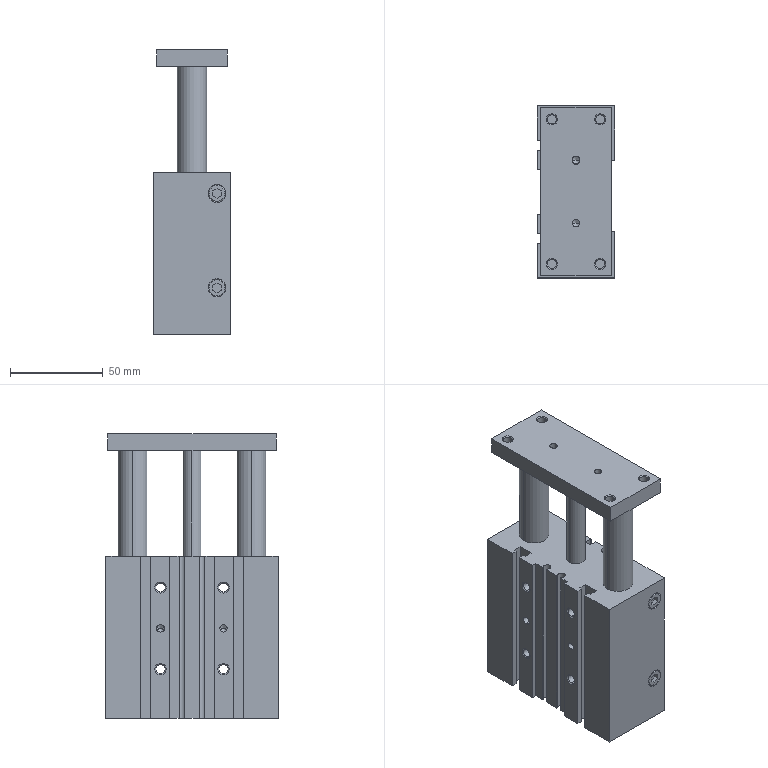Part | SolidWorks | 6 solids | 330 faces | box 42 x 93 x 153.5 mm | volume 318339 mm3 | plane 132 | cylinder 118 | cone 80 | commonest cylinder face diameters 4.917 x24 4 x18 0.6 x8 5.4 x8 8.566 x8 9.5 x8